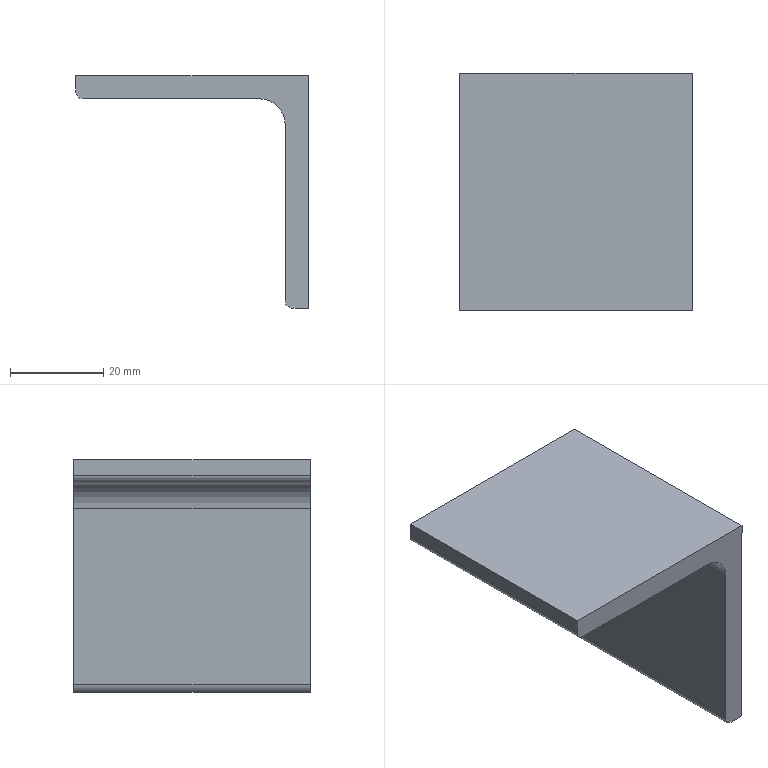Part | SolidWorks | features Fillet 2, Extrusion 1 | 1 solid | 11 faces | box 50 x 50.8 x 50 mm | volume 24399 mm3 | plane 8 | cylinder 3 | commonest cylinder face diameters 3.34 x2 11 x1
STEP:
#1=CARTESIAN_POINT('',(0.,-25.4,-25.));
#2=VERTEX_POINT('',#1);
#3=CARTESIAN_POINT('',(-3.33,-25.4,-25.));
#4=VERTEX_POINT('',#3);
#5=CARTESIAN_POINT('',(0.,-25.4,-25.));
#6=DIRECTION('',(-1.,0.,0.));
#7=VECTOR('',#6,1000.);
#8=LINE('',#5,#7);
#9=EDGE_CURVE('',#2,#4,#8,.T.);
#10=ORIENTED_EDGE('',*,*,#9,.T.);
#11=CARTESIAN_POINT('',(-3.33,25.4,-25.));
#12=VERTEX_POINT('',#11);
#13=CARTESIAN_POINT('',(-3.33,25.4,-25.));
#14=DIRECTION('',(0.,1.,0.));
#15=VECTOR('',#14,1000.);
#16=LINE('',#13,#15);
#17=EDGE_CURVE('',#4,#12,#16,.T.);
#18=ORIENTED_EDGE('',*,*,#17,.T.);
#19=CARTESIAN_POINT('',(0.,25.4,-25.));
#20=VERTEX_POINT('',#19);
#21=CARTESIAN_POINT('',(0.,25.4,-25.));
#22=DIRECTION('',(-1.,0.,0.));
#23=VECTOR('',#22,1000.);
#24=LINE('',#21,#23);
#25=EDGE_CURVE('',#20,#12,#24,.T.);
#26=ORIENTED_EDGE('',*,*,#25,.F.);
#27=CARTESIAN_POINT('',(0.,25.4,-25.));
#28=DIRECTION('',(0.,-1.,0.));
#29=VECTOR('',#28,1000.);
#30=LINE('',#27,#29);
#31=EDGE_CURVE('',#20,#2,#30,.T.);
#32=ORIENTED_EDGE('',*,*,#31,.T.);
#33=EDGE_LOOP('',(#10,#18,#26,#32));
#34=FACE_OUTER_BOUND('',#33,.T.);
#35=CARTESIAN_POINT('',(0.,25.4,-25.));
#36=DIRECTION('',(0.,0.,1.));
#37=DIRECTION('',(1.,0.,0.));
#38=AXIS2_PLACEMENT_3D('',#35,#36,#37);
#39=PLANE('',#38);
#40=ADVANCED_FACE('',(#34),#39,.F.);
#41=CARTESIAN_POINT('',(-5.,25.4,-23.33));
#42=VERTEX_POINT('',#41);
#43=CARTESIAN_POINT('',(-5.,25.4,14.5));
#44=VERTEX_POINT('',#43);
#45=CARTESIAN_POINT('',(-5.,25.4,-25.));
#46=DIRECTION('',(0.,0.,1.));
#47=VECTOR('',#46,1000.);
#48=LINE('',#45,#47);
#49=EDGE_CURVE('',#42,#44,#48,.T.);
#50=ORIENTED_EDGE('',*,*,#49,.F.);
#51=CARTESIAN_POINT('',(-5.,-25.4,-23.33));
#52=VERTEX_POINT('',#51);
#53=CARTESIAN_POINT('',(-5.,25.4,-23.33));
#54=DIRECTION('',(0.,-1.,0.));
#55=VECTOR('',#54,1000.);
#56=LINE('',#53,#55);
#57=EDGE_CURVE('',#42,#52,#56,.T.);
#58=ORIENTED_EDGE('',*,*,#57,.T.);
#59=CARTESIAN_POINT('',(-5.,-25.4,14.5));
#60=VERTEX_POINT('',#59);
#61=CARTESIAN_POINT('',(-5.,-25.4,-25.));
#62=DIRECTION('',(0.,0.,1.));
#63=VECTOR('',#62,1000.);
#64=LINE('',#61,#63);
#65=EDGE_CURVE('',#52,#60,#64,.T.);
#66=ORIENTED_EDGE('',*,*,#65,.T.);
#67=CARTESIAN_POINT('',(-5.,25.4,14.5));
#68=DIRECTION('',(0.,1.,0.));
#69=VECTOR('',#68,1000.);
#70=LINE('',#67,#69);
#71=EDGE_CURVE('',#60,#44,#70,.T.);
#72=ORIENTED_EDGE('',*,*,#71,.T.);
#73=EDGE_LOOP('',(#50,#58,#66,#72));
#74=FACE_OUTER_BOUND('',#73,.T.);
#75=CARTESIAN_POINT('',(-5.,25.4,-25.));
#76=DIRECTION('',(1.,0.,0.));
#77=DIRECTION('',(0.,0.,-1.));
#78=AXIS2_PLACEMENT_3D('',#75,#76,#77);
#79=PLANE('',#78);
#80=ADVANCED_FACE('',(#74),#79,.F.);
#81=CARTESIAN_POINT('',(-10.5,-25.4,20.));
#82=VERTEX_POINT('',#81);
#83=CARTESIAN_POINT('',(-48.33,-25.4,20.));
#84=VERTEX_POINT('',#83);
#85=CARTESIAN_POINT('',(-5.,-25.4,20.));
#86=DIRECTION('',(-1.,0.,0.));
#87=VECTOR('',#86,1000.);
#88=LINE('',#85,#87);
#89=EDGE_CURVE('',#82,#84,#88,.T.);
#90=ORIENTED_EDGE('',*,*,#89,.T.);
#91=CARTESIAN_POINT('',(-48.33,25.4,20.));
#92=VERTEX_POINT('',#91);
#93=CARTESIAN_POINT('',(-48.33,25.4,20.));
#94=DIRECTION('',(0.,1.,0.));
#95=VECTOR('',#94,1000.);
#96=LINE('',#93,#95);
#97=EDGE_CURVE('',#84,#92,#96,.T.);
#98=ORIENTED_EDGE('',*,*,#97,.T.);
#99=CARTESIAN_POINT('',(-10.5,25.4,20.));
#100=VERTEX_POINT('',#99);
#101=CARTESIAN_POINT('',(-5.,25.4,20.));
#102=DIRECTION('',(-1.,0.,0.));
#103=VECTOR('',#102,1000.);
#104=LINE('',#101,#103);
#105=EDGE_CURVE('',#100,#92,#104,.T.);
#106=ORIENTED_EDGE('',*,*,#105,.F.);
#107=CARTESIAN_POINT('',(-10.5,-25.4,20.));
#108=DIRECTION('',(0.,-1.,0.));
#109=VECTOR('',#108,1000.);
#110=LINE('',#107,#109);
#111=EDGE_CURVE('',#100,#82,#110,.T.);
#112=ORIENTED_EDGE('',*,*,#111,.T.);
#113=EDGE_LOOP('',(#90,#98,#106,#112));
#114=FACE_OUTER_BOUND('',#113,.T.);
#115=CARTESIAN_POINT('',(-5.,25.4,20.));
#116=DIRECTION('',(0.,0.,1.));
#117=DIRECTION('',(1.,0.,0.));
#118=AXIS2_PLACEMENT_3D('',#115,#116,#117);
#119=PLANE('',#118);
#120=ADVANCED_FACE('',(#114),#119,.F.);
#121=CARTESIAN_POINT('',(-50.,25.4,21.67));
#122=VERTEX_POINT('',#121);
#123=CARTESIAN_POINT('',(-50.,25.4,25.));
#124=VERTEX_POINT('',#123);
#125=CARTESIAN_POINT('',(-50.,25.4,20.));
#126=DIRECTION('',(0.,0.,1.));
#127=VECTOR('',#126,1000.);
#128=LINE('',#125,#127);
#129=EDGE_CURVE('',#122,#124,#128,.T.);
#130=ORIENTED_EDGE('',*,*,#129,.F.);
#131=CARTESIAN_POINT('',(-50.,-25.4,21.67));
#132=VERTEX_POINT('',#131);
#133=CARTESIAN_POINT('',(-50.,25.4,21.67));
#134=DIRECTION('',(0.,-1.,0.));
#135=VECTOR('',#134,1000.);
#136=LINE('',#133,#135);
#137=EDGE_CURVE('',#122,#132,#136,.T.);
#138=ORIENTED_EDGE('',*,*,#137,.T.);
#139=CARTESIAN_POINT('',(-50.,-25.4,25.));
#140=VERTEX_POINT('',#139);
#141=CARTESIAN_POINT('',(-50.,-25.4,20.));
#142=DIRECTION('',(0.,0.,1.));
#143=VECTOR('',#142,1000.);
#144=LINE('',#141,#143);
#145=EDGE_CURVE('',#132,#140,#144,.T.);
#146=ORIENTED_EDGE('',*,*,#145,.T.);
#147=CARTESIAN_POINT('',(-50.,25.4,25.));
#148=DIRECTION('',(0.,-1.,0.));
#149=VECTOR('',#148,1000.);
#150=LINE('',#147,#149);
#151=EDGE_CURVE('',#124,#140,#150,.T.);
#152=ORIENTED_EDGE('',*,*,#151,.F.);
#153=EDGE_LOOP('',(#130,#138,#146,#152));
#154=FACE_OUTER_BOUND('',#153,.T.);
#155=CARTESIAN_POINT('',(-50.,25.4,20.));
#156=DIRECTION('',(1.,0.,0.));
#157=DIRECTION('',(0.,0.,-1.));
#158=AXIS2_PLACEMENT_3D('',#155,#156,#157);
#159=PLANE('',#158);
#160=ADVANCED_FACE('',(#154),#159,.F.);
#161=CARTESIAN_POINT('',(0.,-25.4,25.));
#162=VERTEX_POINT('',#161);
#163=CARTESIAN_POINT('',(-50.,-25.4,25.));
#164=DIRECTION('',(1.,0.,0.));
#165=VECTOR('',#164,1000.);
#166=LINE('',#163,#165);
#167=EDGE_CURVE('',#140,#162,#166,.T.);
#168=ORIENTED_EDGE('',*,*,#167,.T.);
#169=CARTESIAN_POINT('',(0.,25.4,25.));
#170=VERTEX_POINT('',#169);
#171=CARTESIAN_POINT('',(0.,25.4,25.));
#172=DIRECTION('',(0.,-1.,0.));
#173=VECTOR('',#172,1000.);
#174=LINE('',#171,#173);
#175=EDGE_CURVE('',#170,#162,#174,.T.);
#176=ORIENTED_EDGE('',*,*,#175,.F.);
#177=CARTESIAN_POINT('',(-50.,25.4,25.));
#178=DIRECTION('',(1.,0.,0.));
#179=VECTOR('',#178,1000.);
#180=LINE('',#177,#179);
#181=EDGE_CURVE('',#124,#170,#180,.T.);
#182=ORIENTED_EDGE('',*,*,#181,.F.);
#183=ORIENTED_EDGE('',*,*,#151,.T.);
#184=EDGE_LOOP('',(#168,#176,#182,#183));
#185=FACE_OUTER_BOUND('',#184,.T.);
#186=CARTESIAN_POINT('',(-50.,25.4,25.));
#187=DIRECTION('',(0.,0.,-1.));
#188=DIRECTION('',(-1.,0.,0.));
#189=AXIS2_PLACEMENT_3D('',#186,#187,#188);
#190=PLANE('',#189);
#191=ADVANCED_FACE('',(#185),#190,.F.);
#192=CARTESIAN_POINT('',(0.,-25.4,25.));
#193=DIRECTION('',(0.,0.,-1.));
#194=VECTOR('',#193,1000.);
#195=LINE('',#192,#194);
#196=EDGE_CURVE('',#162,#2,#195,.T.);
#197=ORIENTED_EDGE('',*,*,#196,.T.);
#198=ORIENTED_EDGE('',*,*,#31,.F.);
#199=CARTESIAN_POINT('',(0.,25.4,25.));
#200=DIRECTION('',(0.,0.,-1.));
#201=VECTOR('',#200,1000.);
#202=LINE('',#199,#201);
#203=EDGE_CURVE('',#170,#20,#202,.T.);
#204=ORIENTED_EDGE('',*,*,#203,.F.);
#205=ORIENTED_EDGE('',*,*,#175,.T.);
#206=EDGE_LOOP('',(#197,#198,#204,#205));
#207=FACE_OUTER_BOUND('',#206,.T.);
#208=CARTESIAN_POINT('',(0.,25.4,25.));
#209=DIRECTION('',(-1.,0.,0.));
#210=DIRECTION('',(0.,0.,1.));
#211=AXIS2_PLACEMENT_3D('',#208,#209,#210);
#212=PLANE('',#211);
#213=ADVANCED_FACE('',(#207),#212,.F.);
#214=ORIENTED_EDGE('',*,*,#105,.T.);
#215=CARTESIAN_POINT('',(-48.33,25.4,21.67));
#216=DIRECTION('',(0.,1.,0.));
#217=DIRECTION('',(0.,0.,-1.));
#218=AXIS2_PLACEMENT_3D('',#215,#216,#217);
#219=CIRCLE('',#218,1.67);
#220=EDGE_CURVE('',#92,#122,#219,.T.);
#221=ORIENTED_EDGE('',*,*,#220,.T.);
#222=ORIENTED_EDGE('',*,*,#129,.T.);
#223=ORIENTED_EDGE('',*,*,#181,.T.);
#224=ORIENTED_EDGE('',*,*,#203,.T.);
#225=ORIENTED_EDGE('',*,*,#25,.T.);
#226=CARTESIAN_POINT('',(-3.33,25.4,-23.33));
#227=DIRECTION('',(0.,1.,0.));
#228=DIRECTION('',(0.,0.,-1.));
#229=AXIS2_PLACEMENT_3D('',#226,#227,#228);
#230=CIRCLE('',#229,1.67);
#231=EDGE_CURVE('',#12,#42,#230,.T.);
#232=ORIENTED_EDGE('',*,*,#231,.T.);
#233=ORIENTED_EDGE('',*,*,#49,.T.);
#234=CARTESIAN_POINT('',(-10.5,25.4,14.5));
#235=DIRECTION('',(0.,-1.,0.));
#236=DIRECTION('',(0.,0.,-1.));
#237=AXIS2_PLACEMENT_3D('',#234,#235,#236);
#238=CIRCLE('',#237,5.5);
#239=EDGE_CURVE('',#44,#100,#238,.T.);
#240=ORIENTED_EDGE('',*,*,#239,.T.);
#241=EDGE_LOOP('',(#214,#221,#222,#223,#224,#225,#232,#233,#240));
#242=FACE_OUTER_BOUND('',#241,.T.);
#243=CARTESIAN_POINT('',(0.,25.4,-25.));
#244=DIRECTION('',(0.,-1.,0.));
#245=DIRECTION('',(0.,0.,-1.));
#246=AXIS2_PLACEMENT_3D('',#243,#244,#245);
#247=PLANE('',#246);
#248=ADVANCED_FACE('',(#242),#247,.F.);
#249=ORIENTED_EDGE('',*,*,#145,.F.);
#250=CARTESIAN_POINT('',(-48.33,-25.4,21.67));
#251=DIRECTION('',(0.,-1.,0.));
#252=DIRECTION('',(0.,0.,-1.));
#253=AXIS2_PLACEMENT_3D('',#250,#251,#252);
#254=CIRCLE('',#253,1.67);
#255=EDGE_CURVE('',#132,#84,#254,.T.);
#256=ORIENTED_EDGE('',*,*,#255,.T.);
#257=ORIENTED_EDGE('',*,*,#89,.F.);
#258=CARTESIAN_POINT('',(-10.5,-25.4,14.5));
#259=DIRECTION('',(0.,1.,0.));
#260=DIRECTION('',(0.,0.,-1.));
#261=AXIS2_PLACEMENT_3D('',#258,#259,#260);
#262=CIRCLE('',#261,5.5);
#263=EDGE_CURVE('',#82,#60,#262,.T.);
#264=ORIENTED_EDGE('',*,*,#263,.T.);
#265=ORIENTED_EDGE('',*,*,#65,.F.);
#266=CARTESIAN_POINT('',(-3.33,-25.4,-23.33));
#267=DIRECTION('',(0.,-1.,0.));
#268=DIRECTION('',(0.,0.,-1.));
#269=AXIS2_PLACEMENT_3D('',#266,#267,#268);
#270=CIRCLE('',#269,1.67);
#271=EDGE_CURVE('',#52,#4,#270,.T.);
#272=ORIENTED_EDGE('',*,*,#271,.T.);
#273=ORIENTED_EDGE('',*,*,#9,.F.);
#274=ORIENTED_EDGE('',*,*,#196,.F.);
#275=ORIENTED_EDGE('',*,*,#167,.F.);
#276=EDGE_LOOP('',(#249,#256,#257,#264,#265,#272,#273,#274,#275));
#277=FACE_OUTER_BOUND('',#276,.T.);
#278=CARTESIAN_POINT('',(0.,-25.4,-25.));
#279=DIRECTION('',(0.,-1.,0.));
#280=DIRECTION('',(0.,0.,-1.));
#281=AXIS2_PLACEMENT_3D('',#278,#279,#280);
#282=PLANE('',#281);
#283=ADVANCED_FACE('',(#277),#282,.T.);
#284=ORIENTED_EDGE('',*,*,#239,.F.);
#285=ORIENTED_EDGE('',*,*,#71,.F.);
#286=ORIENTED_EDGE('',*,*,#263,.F.);
#287=ORIENTED_EDGE('',*,*,#111,.F.);
#288=EDGE_LOOP('',(#284,#285,#286,#287));
#289=FACE_OUTER_BOUND('',#288,.T.);
#290=CARTESIAN_POINT('',(-10.5,25.4,14.5));
#291=DIRECTION('',(0.,1.,0.));
#292=DIRECTION('',(0.,0.,1.));
#293=AXIS2_PLACEMENT_3D('',#290,#291,#292);
#294=CYLINDRICAL_SURFACE('',#293,5.5);
#295=ADVANCED_FACE('',(#289),#294,.F.);
#296=ORIENTED_EDGE('',*,*,#220,.F.);
#297=ORIENTED_EDGE('',*,*,#97,.F.);
#298=ORIENTED_EDGE('',*,*,#255,.F.);
#299=ORIENTED_EDGE('',*,*,#137,.F.);
#300=EDGE_LOOP('',(#296,#297,#298,#299));
#301=FACE_OUTER_BOUND('',#300,.T.);
#302=CARTESIAN_POINT('',(-48.33,25.4,21.67));
#303=DIRECTION('',(0.,-1.,0.));
#304=DIRECTION('',(0.,0.,-1.));
#305=AXIS2_PLACEMENT_3D('',#302,#303,#304);
#306=CYLINDRICAL_SURFACE('',#305,1.67);
#307=ADVANCED_FACE('',(#301),#306,.T.);
#308=ORIENTED_EDGE('',*,*,#231,.F.);
#309=ORIENTED_EDGE('',*,*,#17,.F.);
#310=ORIENTED_EDGE('',*,*,#271,.F.);
#311=ORIENTED_EDGE('',*,*,#57,.F.);
#312=EDGE_LOOP('',(#308,#309,#310,#311));
#313=FACE_OUTER_BOUND('',#312,.T.);
#314=CARTESIAN_POINT('',(-3.33,25.4,-23.33));
#315=DIRECTION('',(0.,-1.,0.));
#316=DIRECTION('',(0.,0.,-1.));
#317=AXIS2_PLACEMENT_3D('',#314,#315,#316);
#318=CYLINDRICAL_SURFACE('',#317,1.67);
#319=ADVANCED_FACE('',(#313),#318,.T.);
#320=CLOSED_SHELL('',(#40,#80,#120,#160,#191,#213,#248,#283,#295,#307,#319));
#321=MANIFOLD_SOLID_BREP('',#320);
#322=CARTESIAN_POINT('',(0.,0.,0.));
#323=DIRECTION('',(0.,0.,1.));
#324=DIRECTION('',(1.,0.,0.));
#325=AXIS2_PLACEMENT_3D('',#322,#323,#324);
#326=(LENGTH_UNIT()NAMED_UNIT(*)SI_UNIT(.MILLI.,.METRE.));
#327=UNCERTAINTY_MEASURE_WITH_UNIT(LENGTH_MEASURE(0.00001),#326,'','');
#328=(NAMED_UNIT(*)PLANE_ANGLE_UNIT()SI_UNIT($,.RADIAN.));
#329=(NAMED_UNIT(*)SI_UNIT($,.STERADIAN.)SOLID_ANGLE_UNIT());
#330=(GEOMETRIC_REPRESENTATION_CONTEXT(3)GLOBAL_UNCERTAINTY_ASSIGNED_CONTEXT((#327))GLOBAL_UNIT_ASSIGNED_CONTEXT((#326,#328,#329))REPRESENTATION_CONTEXT('',''));
#331=ADVANCED_BREP_SHAPE_REPRESENTATION('',(#321,#325),#330);